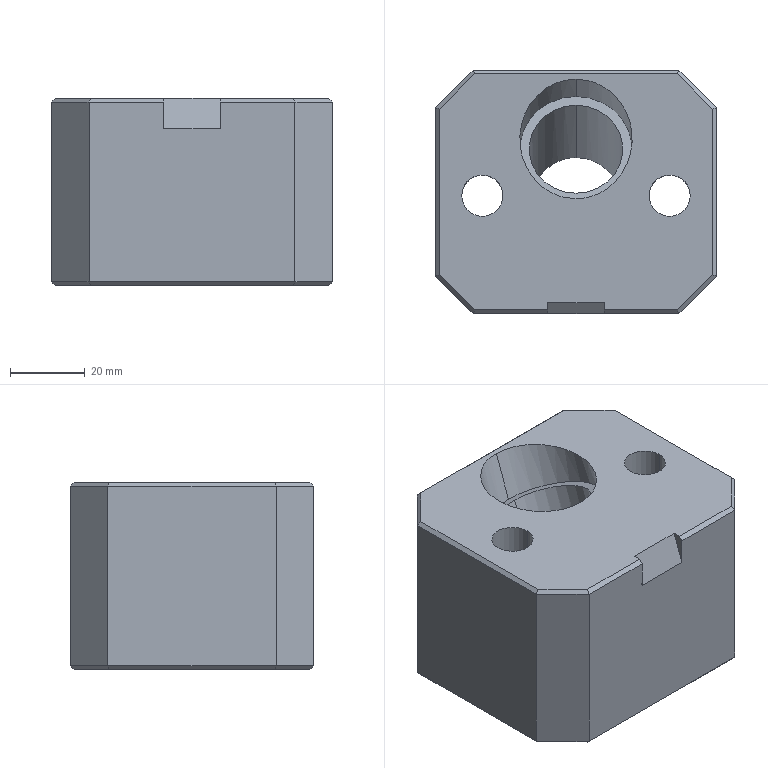Part | Creo | 3 solids | 49 faces | box 75 x 65 x 50 mm | volume 192479 mm3 | plane 33 | cylinder 16 | commonest cylinder face diameters 11 x4 18 x4 11.98 x2 12 x2 25 x2 30 x2
STEP:
#1=CARTESIAN_POINT('',(0.,-322.338,40.));
#2=VERTEX_POINT('',#1);
#3=CARTESIAN_POINT('',(0.,-290.412,40.));
#4=VERTEX_POINT('',#3);
#5=CARTESIAN_POINT('',(0.,-322.338,40.));
#6=CARTESIAN_POINT('',(-1.768,-322.338,40.));
#7=CARTESIAN_POINT('',(-5.588,-321.656,40.));
#8=CARTESIAN_POINT('',(-10.029,-318.608,40.));
#9=CARTESIAN_POINT('',(-12.65,-315.161,40.));
#10=CARTESIAN_POINT('',(-14.047,-312.268,40.));
#11=CARTESIAN_POINT('',(-14.71,-309.769,40.));
#12=CARTESIAN_POINT('',(-14.961,-307.801,40.));
#13=CARTESIAN_POINT('',(-15.02,-306.375,40.));
#14=CARTESIAN_POINT('',(-14.961,-304.949,40.));
#15=CARTESIAN_POINT('',(-14.71,-302.981,40.));
#16=CARTESIAN_POINT('',(-14.047,-300.481,40.));
#17=CARTESIAN_POINT('',(-12.65,-297.589,40.));
#18=CARTESIAN_POINT('',(-10.029,-294.142,40.));
#19=CARTESIAN_POINT('',(-5.588,-291.094,40.));
#20=CARTESIAN_POINT('',(-1.768,-290.412,40.));
#21=CARTESIAN_POINT('',(0.,-290.412,40.));
#22=B_SPLINE_CURVE_WITH_KNOTS('',3,(#5,#6,#7,#8,#9,#10,#11,#12,#13,#14,#15,#16,#17,#18,#19,#20,#21),.UNSPECIFIED.,.F.,.F.,(4,1,1,1,1,1,1,1,1,1,1,1,1,1,4),(0.,0.125,0.25,0.3125,0.375,0.4375,0.4688,0.5,0.5312,0.5625,0.625,0.6875,0.75,0.875,1.),.UNSPECIFIED.);
#23=EDGE_CURVE('',#2,#4,#22,.T.);
#24=ORIENTED_EDGE('',*,*,#23,.T.);
#25=CARTESIAN_POINT('',(0.,-295.009,27.371));
#26=VERTEX_POINT('',#25);
#27=CARTESIAN_POINT('',(0.,-290.412,40.));
#28=DIRECTION('',(0.,-0.342,-0.9397));
#29=VECTOR('',#28,13.44);
#30=LINE('',#27,#29);
#31=EDGE_CURVE('',#4,#26,#30,.T.);
#32=ORIENTED_EDGE('',*,*,#31,.T.);
#33=CARTESIAN_POINT('',(0.,-323.2,37.631));
#34=VERTEX_POINT('',#33);
#35=CARTESIAN_POINT('',(0.,-309.104,32.501));
#36=DIRECTION('',(0.,0.342,0.9397));
#37=DIRECTION('',(0.,0.9397,-0.342));
#38=AXIS2_PLACEMENT_3D('',#35,#36,#37);
#39=CIRCLE('',#38,15.);
#40=EDGE_CURVE('',#26,#34,#39,.T.);
#41=ORIENTED_EDGE('',*,*,#40,.T.);
#42=CARTESIAN_POINT('',(0.,-322.338,40.));
#43=DIRECTION('',(0.,-0.342,-0.9397));
#44=VECTOR('',#43,2.521);
#45=LINE('',#42,#44);
#46=EDGE_CURVE('',#2,#34,#45,.T.);
#47=ORIENTED_EDGE('',*,*,#46,.F.);
#48=EDGE_LOOP('',(#24,#32,#41,#47));
#49=FACE_OUTER_BOUND('',#48,.F.);
#50=CARTESIAN_POINT('',(0.,-302.52,50.59));
#51=DIRECTION('',(0.,-0.342,-0.9397));
#52=DIRECTION('',(0.,-0.9397,0.342));
#53=AXIS2_PLACEMENT_3D('',#50,#51,#52);
#54=CYLINDRICAL_SURFACE('',#53,15.);
#55=ADVANCED_FACE('',(#49),#54,.F.);
#56=CARTESIAN_POINT('',(-7.502,-352.,40.));
#57=VERTEX_POINT('',#56);
#58=CARTESIAN_POINT('',(-7.502,-350.064,40.));
#59=VERTEX_POINT('',#58);
#60=CARTESIAN_POINT('',(-7.502,-352.,40.));
#61=DIRECTION('',(0.,1.,0.));
#62=VECTOR('',#61,1.936);
#63=LINE('',#60,#62);
#64=EDGE_CURVE('',#57,#59,#63,.T.);
#65=ORIENTED_EDGE('',*,*,#64,.F.);
#66=CARTESIAN_POINT('',(-27.087,-352.,40.));
#67=VERTEX_POINT('',#66);
#68=CARTESIAN_POINT('',(-7.502,-352.,40.));
#69=DIRECTION('',(-1.,0.,0.));
#70=VECTOR('',#69,19.586);
#71=LINE('',#68,#70);
#72=EDGE_CURVE('',#57,#67,#71,.T.);
#73=ORIENTED_EDGE('',*,*,#72,.T.);
#74=CARTESIAN_POINT('',(-36.502,-342.586,40.));
#75=VERTEX_POINT('',#74);
#76=CARTESIAN_POINT('',(-36.502,-342.586,40.));
#77=DIRECTION('',(0.7071,-0.7071,0.));
#78=VECTOR('',#77,13.314);
#79=LINE('',#76,#78);
#80=EDGE_CURVE('',#75,#67,#79,.T.);
#81=ORIENTED_EDGE('',*,*,#80,.F.);
#82=CARTESIAN_POINT('',(-36.502,-298.414,40.));
#83=VERTEX_POINT('',#82);
#84=CARTESIAN_POINT('',(-36.502,-342.586,40.));
#85=DIRECTION('',(0.,1.,0.));
#86=VECTOR('',#85,44.172);
#87=LINE('',#84,#86);
#88=EDGE_CURVE('',#75,#83,#87,.T.);
#89=ORIENTED_EDGE('',*,*,#88,.T.);
#90=CARTESIAN_POINT('',(-27.087,-289.,40.));
#91=VERTEX_POINT('',#90);
#92=CARTESIAN_POINT('',(-27.087,-289.,40.));
#93=DIRECTION('',(-0.7071,-0.7071,0.));
#94=VECTOR('',#93,13.314);
#95=LINE('',#92,#94);
#96=EDGE_CURVE('',#91,#83,#95,.T.);
#97=ORIENTED_EDGE('',*,*,#96,.F.);
#98=CARTESIAN_POINT('',(27.084,-289.,40.));
#99=VERTEX_POINT('',#98);
#100=CARTESIAN_POINT('',(-27.087,-289.,40.));
#101=DIRECTION('',(1.,0.,0.));
#102=VECTOR('',#101,54.172);
#103=LINE('',#100,#102);
#104=EDGE_CURVE('',#91,#99,#103,.T.);
#105=ORIENTED_EDGE('',*,*,#104,.T.);
#106=CARTESIAN_POINT('',(36.498,-298.414,40.));
#107=VERTEX_POINT('',#106);
#108=CARTESIAN_POINT('',(36.498,-298.414,40.));
#109=DIRECTION('',(-0.7071,0.7071,0.));
#110=VECTOR('',#109,13.314);
#111=LINE('',#108,#110);
#112=EDGE_CURVE('',#107,#99,#111,.T.);
#113=ORIENTED_EDGE('',*,*,#112,.F.);
#114=CARTESIAN_POINT('',(36.498,-342.586,40.));
#115=VERTEX_POINT('',#114);
#116=CARTESIAN_POINT('',(36.498,-298.414,40.));
#117=DIRECTION('',(0.,-1.,0.));
#118=VECTOR('',#117,44.172);
#119=LINE('',#116,#118);
#120=EDGE_CURVE('',#107,#115,#119,.T.);
#121=ORIENTED_EDGE('',*,*,#120,.T.);
#122=CARTESIAN_POINT('',(27.084,-352.,40.));
#123=VERTEX_POINT('',#122);
#124=CARTESIAN_POINT('',(27.084,-352.,40.));
#125=DIRECTION('',(0.7071,0.7071,0.));
#126=VECTOR('',#125,13.314);
#127=LINE('',#124,#126);
#128=EDGE_CURVE('',#123,#115,#127,.T.);
#129=ORIENTED_EDGE('',*,*,#128,.F.);
#130=CARTESIAN_POINT('',(7.498,-352.,40.));
#131=VERTEX_POINT('',#130);
#132=CARTESIAN_POINT('',(27.084,-352.,40.));
#133=DIRECTION('',(-1.,0.,0.));
#134=VECTOR('',#133,19.586);
#135=LINE('',#132,#134);
#136=EDGE_CURVE('',#123,#131,#135,.T.);
#137=ORIENTED_EDGE('',*,*,#136,.T.);
#138=CARTESIAN_POINT('',(7.498,-350.064,40.));
#139=VERTEX_POINT('',#138);
#140=CARTESIAN_POINT('',(7.498,-350.064,40.));
#141=DIRECTION('',(0.,-1.,0.));
#142=VECTOR('',#141,1.936);
#143=LINE('',#140,#142);
#144=EDGE_CURVE('',#139,#131,#143,.T.);
#145=ORIENTED_EDGE('',*,*,#144,.F.);
#146=CARTESIAN_POINT('',(-7.502,-350.064,40.));
#147=DIRECTION('',(1.,0.,0.));
#148=VECTOR('',#147,15.);
#149=LINE('',#146,#148);
#150=EDGE_CURVE('',#59,#139,#149,.T.);
#151=ORIENTED_EDGE('',*,*,#150,.F.);
#152=EDGE_LOOP('',(#65,#73,#81,#89,#97,#105,#113,#121,#129,#137,#145,#151));
#153=FACE_OUTER_BOUND('',#152,.F.);
#154=CARTESIAN_POINT('',(-19.502,-321.5,40.));
#155=VERTEX_POINT('',#154);
#156=CARTESIAN_POINT('',(-30.502,-321.5,40.));
#157=VERTEX_POINT('',#156);
#158=CARTESIAN_POINT('',(-25.002,-321.5,40.));
#159=DIRECTION('',(0.,0.,-1.));
#160=DIRECTION('',(1.,0.,0.));
#161=AXIS2_PLACEMENT_3D('',#158,#159,#160);
#162=CIRCLE('',#161,5.5);
#163=EDGE_CURVE('',#155,#157,#162,.T.);
#164=ORIENTED_EDGE('',*,*,#163,.F.);
#165=CARTESIAN_POINT('',(-25.002,-321.5,40.));
#166=DIRECTION('',(0.,0.,-1.));
#167=DIRECTION('',(-1.,0.,0.));
#168=AXIS2_PLACEMENT_3D('',#165,#166,#167);
#169=CIRCLE('',#168,5.5);
#170=EDGE_CURVE('',#157,#155,#169,.T.);
#171=ORIENTED_EDGE('',*,*,#170,.F.);
#172=EDGE_LOOP('',(#164,#171));
#173=FACE_BOUND('',#172,.F.);
#174=CARTESIAN_POINT('',(30.498,-321.5,40.));
#175=VERTEX_POINT('',#174);
#176=CARTESIAN_POINT('',(19.498,-321.5,40.));
#177=VERTEX_POINT('',#176);
#178=CARTESIAN_POINT('',(24.998,-321.5,40.));
#179=DIRECTION('',(0.,0.,-1.));
#180=DIRECTION('',(1.,0.,0.));
#181=AXIS2_PLACEMENT_3D('',#178,#179,#180);
#182=CIRCLE('',#181,5.5);
#183=EDGE_CURVE('',#175,#177,#182,.T.);
#184=ORIENTED_EDGE('',*,*,#183,.F.);
#185=CARTESIAN_POINT('',(24.998,-321.5,40.));
#186=DIRECTION('',(0.,0.,-1.));
#187=DIRECTION('',(-1.,0.,0.));
#188=AXIS2_PLACEMENT_3D('',#185,#186,#187);
#189=CIRCLE('',#188,5.5);
#190=EDGE_CURVE('',#177,#175,#189,.T.);
#191=ORIENTED_EDGE('',*,*,#190,.F.);
#192=EDGE_LOOP('',(#184,#191));
#193=FACE_BOUND('',#192,.F.);
#194=ORIENTED_EDGE('',*,*,#23,.F.);
#195=CARTESIAN_POINT('',(0.,-290.412,40.));
#196=CARTESIAN_POINT('',(1.768,-290.412,40.));
#197=CARTESIAN_POINT('',(5.588,-291.094,40.));
#198=CARTESIAN_POINT('',(10.029,-294.142,40.));
#199=CARTESIAN_POINT('',(12.65,-297.589,40.));
#200=CARTESIAN_POINT('',(14.047,-300.481,40.));
#201=CARTESIAN_POINT('',(14.71,-302.981,40.));
#202=CARTESIAN_POINT('',(14.961,-304.949,40.));
#203=CARTESIAN_POINT('',(15.02,-306.375,40.));
#204=CARTESIAN_POINT('',(14.961,-307.801,40.));
#205=CARTESIAN_POINT('',(14.71,-309.769,40.));
#206=CARTESIAN_POINT('',(14.047,-312.268,40.));
#207=CARTESIAN_POINT('',(12.65,-315.161,40.));
#208=CARTESIAN_POINT('',(10.029,-318.608,40.));
#209=CARTESIAN_POINT('',(5.588,-321.656,40.));
#210=CARTESIAN_POINT('',(1.768,-322.338,40.));
#211=CARTESIAN_POINT('',(0.,-322.338,40.));
#212=B_SPLINE_CURVE_WITH_KNOTS('',3,(#195,#196,#197,#198,#199,#200,#201,#202,#203,#204,#205,#206,#207,#208,#209,#210,#211),.UNSPECIFIED.,.F.,.F.,(4,1,1,1,1,1,1,1,1,1,1,1,1,1,4),(0.,0.125,0.25,0.3125,0.375,0.4375,0.4688,0.5,0.5312,0.5625,0.625,0.6875,0.75,0.875,1.),.UNSPECIFIED.);
#213=EDGE_CURVE('',#4,#2,#212,.T.);
#214=ORIENTED_EDGE('',*,*,#213,.F.);
#215=EDGE_LOOP('',(#194,#214));
#216=FACE_BOUND('',#215,.F.);
#217=CARTESIAN_POINT('',(365.934,-307.397,40.));
#218=DIRECTION('',(0.,0.,1.));
#219=DIRECTION('',(-1.,0.,0.));
#220=AXIS2_PLACEMENT_3D('',#217,#218,#219);
#221=PLANE('',#220);
#222=ADVANCED_FACE('',(#153,#173,#193,#216),#221,.T.);
#223=ORIENTED_EDGE('',*,*,#64,.T.);
#224=CARTESIAN_POINT('',(-7.502,-353.,31.933));
#225=VERTEX_POINT('',#224);
#226=CARTESIAN_POINT('',(-7.502,-353.,31.933));
#227=DIRECTION('',(0.,0.342,0.9397));
#228=VECTOR('',#227,8.584);
#229=LINE('',#226,#228);
#230=EDGE_CURVE('',#225,#59,#229,.T.);
#231=ORIENTED_EDGE('',*,*,#230,.F.);
#232=CARTESIAN_POINT('',(-7.502,-353.,39.));
#233=VERTEX_POINT('',#232);
#234=CARTESIAN_POINT('',(-7.502,-353.,31.933));
#235=DIRECTION('',(0.,0.,1.));
#236=VECTOR('',#235,7.067);
#237=LINE('',#234,#236);
#238=EDGE_CURVE('',#225,#233,#237,.T.);
#239=ORIENTED_EDGE('',*,*,#238,.T.);
#240=CARTESIAN_POINT('',(-7.502,-352.,40.));
#241=DIRECTION('',(0.,-0.7071,-0.7071));
#242=VECTOR('',#241,1.414);
#243=LINE('',#240,#242);
#244=EDGE_CURVE('',#57,#233,#243,.T.);
#245=ORIENTED_EDGE('',*,*,#244,.F.);
#246=EDGE_LOOP('',(#223,#231,#239,#245));
#247=FACE_OUTER_BOUND('',#246,.F.);
#248=CARTESIAN_POINT('',(-7.502,-370.58,-2.601));
#249=DIRECTION('',(-1.,0.,0.));
#250=DIRECTION('',(0.,0.,1.));
#251=AXIS2_PLACEMENT_3D('',#248,#249,#250);
#252=PLANE('',#251);
#253=ADVANCED_FACE('',(#247),#252,.F.);
#254=ORIENTED_EDGE('',*,*,#150,.T.);
#255=CARTESIAN_POINT('',(7.498,-353.,31.933));
#256=VERTEX_POINT('',#255);
#257=CARTESIAN_POINT('',(7.498,-350.064,40.));
#258=DIRECTION('',(0.,-0.342,-0.9397));
#259=VECTOR('',#258,8.584);
#260=LINE('',#257,#259);
#261=EDGE_CURVE('',#139,#256,#260,.T.);
#262=ORIENTED_EDGE('',*,*,#261,.T.);
#263=CARTESIAN_POINT('',(7.498,-353.,31.933));
#264=DIRECTION('',(-1.,0.,0.));
#265=VECTOR('',#264,15.);
#266=LINE('',#263,#265);
#267=EDGE_CURVE('',#256,#225,#266,.T.);
#268=ORIENTED_EDGE('',*,*,#267,.T.);
#269=ORIENTED_EDGE('',*,*,#230,.T.);
#270=EDGE_LOOP('',(#254,#262,#268,#269));
#271=FACE_OUTER_BOUND('',#270,.F.);
#272=CARTESIAN_POINT('',(-0.00154,-366.156,-4.212));
#273=DIRECTION('',(0.,0.9397,-0.342));
#274=DIRECTION('',(0.,0.342,0.9397));
#275=AXIS2_PLACEMENT_3D('',#272,#273,#274);
#276=PLANE('',#275);
#277=ADVANCED_FACE('',(#271),#276,.F.);
#278=ORIENTED_EDGE('',*,*,#144,.T.);
#279=CARTESIAN_POINT('',(7.498,-353.,39.));
#280=VERTEX_POINT('',#279);
#281=CARTESIAN_POINT('',(7.498,-353.,39.));
#282=DIRECTION('',(0.,0.7071,0.7071));
#283=VECTOR('',#282,1.414);
#284=LINE('',#281,#283);
#285=EDGE_CURVE('',#280,#131,#284,.T.);
#286=ORIENTED_EDGE('',*,*,#285,.F.);
#287=CARTESIAN_POINT('',(7.498,-353.,39.));
#288=DIRECTION('',(0.,0.,-1.));
#289=VECTOR('',#288,7.067);
#290=LINE('',#287,#289);
#291=EDGE_CURVE('',#280,#256,#290,.T.);
#292=ORIENTED_EDGE('',*,*,#291,.T.);
#293=ORIENTED_EDGE('',*,*,#261,.F.);
#294=EDGE_LOOP('',(#278,#286,#292,#293));
#295=FACE_OUTER_BOUND('',#294,.F.);
#296=CARTESIAN_POINT('',(7.498,-370.58,-2.601));
#297=DIRECTION('',(1.,0.,0.));
#298=DIRECTION('',(0.,0.,-1.));
#299=AXIS2_PLACEMENT_3D('',#296,#297,#298);
#300=PLANE('',#299);
#301=ADVANCED_FACE('',(#295),#300,.F.);
#302=ORIENTED_EDGE('',*,*,#285,.T.);
#303=ORIENTED_EDGE('',*,*,#136,.F.);
#304=CARTESIAN_POINT('',(27.498,-353.,39.));
#305=VERTEX_POINT('',#304);
#306=CARTESIAN_POINT('',(27.498,-353.,39.));
#307=DIRECTION('',(-0.2811,0.6786,0.6786));
#308=VECTOR('',#307,1.474);
#309=LINE('',#306,#308);
#310=EDGE_CURVE('',#305,#123,#309,.T.);
#311=ORIENTED_EDGE('',*,*,#310,.F.);
#312=CARTESIAN_POINT('',(7.498,-353.,39.));
#313=DIRECTION('',(1.,0.,0.));
#314=VECTOR('',#313,20.);
#315=LINE('',#312,#314);
#316=EDGE_CURVE('',#280,#305,#315,.T.);
#317=ORIENTED_EDGE('',*,*,#316,.F.);
#318=EDGE_LOOP('',(#302,#303,#311,#317));
#319=FACE_OUTER_BOUND('',#318,.F.);
#320=CARTESIAN_POINT('',(365.934,-352.,40.));
#321=DIRECTION('',(0.,0.7071,-0.7071));
#322=DIRECTION('',(1.,0.,0.));
#323=AXIS2_PLACEMENT_3D('',#320,#321,#322);
#324=PLANE('',#323);
#325=ADVANCED_FACE('',(#319),#324,.F.);
#326=ORIENTED_EDGE('',*,*,#128,.T.);
#327=CARTESIAN_POINT('',(37.498,-343.,39.));
#328=VERTEX_POINT('',#327);
#329=CARTESIAN_POINT('',(37.498,-343.,39.));
#330=DIRECTION('',(-0.6786,0.2811,0.6786));
#331=VECTOR('',#330,1.474);
#332=LINE('',#329,#331);
#333=EDGE_CURVE('',#328,#115,#332,.T.);
#334=ORIENTED_EDGE('',*,*,#333,.F.);
#335=CARTESIAN_POINT('',(27.498,-353.,39.));
#336=DIRECTION('',(0.7071,0.7071,0.));
#337=VECTOR('',#336,14.142);
#338=LINE('',#335,#337);
#339=EDGE_CURVE('',#305,#328,#338,.T.);
#340=ORIENTED_EDGE('',*,*,#339,.F.);
#341=ORIENTED_EDGE('',*,*,#310,.T.);
#342=EDGE_LOOP('',(#326,#334,#340,#341));
#343=FACE_OUTER_BOUND('',#342,.F.);
#344=CARTESIAN_POINT('',(218.811,-160.274,40.));
#345=DIRECTION('',(-0.5,0.5,-0.7071));
#346=DIRECTION('',(0.7071,0.7071,0.));
#347=AXIS2_PLACEMENT_3D('',#344,#345,#346);
#348=PLANE('',#347);
#349=ADVANCED_FACE('',(#343),#348,.F.);
#350=ORIENTED_EDGE('',*,*,#333,.T.);
#351=ORIENTED_EDGE('',*,*,#120,.F.);
#352=CARTESIAN_POINT('',(37.498,-298.,39.));
#353=VERTEX_POINT('',#352);
#354=CARTESIAN_POINT('',(37.498,-298.,39.));
#355=DIRECTION('',(-0.6786,-0.2811,0.6786));
#356=VECTOR('',#355,1.474);
#357=LINE('',#354,#356);
#358=EDGE_CURVE('',#353,#107,#357,.T.);
#359=ORIENTED_EDGE('',*,*,#358,.F.);
#360=CARTESIAN_POINT('',(37.498,-343.,39.));
#361=DIRECTION('',(0.,1.,0.));
#362=VECTOR('',#361,45.);
#363=LINE('',#360,#362);
#364=EDGE_CURVE('',#328,#353,#363,.T.);
#365=ORIENTED_EDGE('',*,*,#364,.F.);
#366=EDGE_LOOP('',(#350,#351,#359,#365));
#367=FACE_OUTER_BOUND('',#366,.F.);
#368=CARTESIAN_POINT('',(36.498,-307.397,40.));
#369=DIRECTION('',(0.7071,0.,0.7071));
#370=DIRECTION('',(0.,-1.,0.));
#371=AXIS2_PLACEMENT_3D('',#368,#369,#370);
#372=PLANE('',#371);
#373=ADVANCED_FACE('',(#367),#372,.T.);
#374=ORIENTED_EDGE('',*,*,#358,.T.);
#375=ORIENTED_EDGE('',*,*,#112,.T.);
#376=CARTESIAN_POINT('',(27.498,-288.,39.));
#377=VERTEX_POINT('',#376);
#378=CARTESIAN_POINT('',(27.498,-288.,39.));
#379=DIRECTION('',(-0.2811,-0.6786,0.6786));
#380=VECTOR('',#379,1.474);
#381=LINE('',#378,#380);
#382=EDGE_CURVE('',#377,#99,#381,.T.);
#383=ORIENTED_EDGE('',*,*,#382,.F.);
#384=CARTESIAN_POINT('',(37.498,-298.,39.));
#385=DIRECTION('',(-0.7071,0.7071,0.));
#386=VECTOR('',#385,14.142);
#387=LINE('',#384,#386);
#388=EDGE_CURVE('',#353,#377,#387,.T.);
#389=ORIENTED_EDGE('',*,*,#388,.F.);
#390=EDGE_LOOP('',(#374,#375,#383,#389));
#391=FACE_OUTER_BOUND('',#390,.F.);
#392=CARTESIAN_POINT('',(205.708,-467.624,40.));
#393=DIRECTION('',(-0.5,-0.5,-0.7071));
#394=DIRECTION('',(-0.7071,0.7071,0.));
#395=AXIS2_PLACEMENT_3D('',#392,#393,#394);
#396=PLANE('',#395);
#397=ADVANCED_FACE('',(#391),#396,.F.);
#398=CARTESIAN_POINT('',(-27.502,-288.,39.));
#399=VERTEX_POINT('',#398);
#400=CARTESIAN_POINT('',(-27.502,-288.,39.));
#401=DIRECTION('',(0.2811,-0.6786,0.6786));
#402=VECTOR('',#401,1.474);
#403=LINE('',#400,#402);
#404=EDGE_CURVE('',#399,#91,#403,.T.);
#405=ORIENTED_EDGE('',*,*,#404,.F.);
#406=CARTESIAN_POINT('',(27.498,-288.,39.));
#407=DIRECTION('',(-1.,0.,0.));
#408=VECTOR('',#407,55.);
#409=LINE('',#406,#408);
#410=EDGE_CURVE('',#377,#399,#409,.T.);
#411=ORIENTED_EDGE('',*,*,#410,.F.);
#412=ORIENTED_EDGE('',*,*,#382,.T.);
#413=ORIENTED_EDGE('',*,*,#104,.F.);
#414=EDGE_LOOP('',(#405,#411,#412,#413));
#415=FACE_OUTER_BOUND('',#414,.F.);
#416=CARTESIAN_POINT('',(278.498,-288.,39.));
#417=DIRECTION('',(0.,-0.7071,-0.7071));
#418=DIRECTION('',(1.,0.,0.));
#419=AXIS2_PLACEMENT_3D('',#416,#417,#418);
#420=PLANE('',#419);
#421=ADVANCED_FACE('',(#415),#420,.F.);
#422=ORIENTED_EDGE('',*,*,#404,.T.);
#423=ORIENTED_EDGE('',*,*,#96,.T.);
#424=CARTESIAN_POINT('',(-37.502,-298.,39.));
#425=VERTEX_POINT('',#424);
#426=CARTESIAN_POINT('',(-36.502,-298.414,40.));
#427=DIRECTION('',(-0.6786,0.2811,-0.6786));
#428=VECTOR('',#427,1.474);
#429=LINE('',#426,#428);
#430=EDGE_CURVE('',#83,#425,#429,.T.);
#431=ORIENTED_EDGE('',*,*,#430,.T.);
#432=CARTESIAN_POINT('',(-27.502,-288.,39.));
#433=DIRECTION('',(-0.7071,-0.7071,0.));
#434=VECTOR('',#433,14.142);
#435=LINE('',#432,#434);
#436=EDGE_CURVE('',#399,#425,#435,.T.);
#437=ORIENTED_EDGE('',*,*,#436,.F.);
#438=EDGE_LOOP('',(#422,#423,#431,#437));
#439=FACE_OUTER_BOUND('',#438,.F.);
#440=CARTESIAN_POINT('',(160.225,-101.688,40.));
#441=DIRECTION('',(-0.5,0.5,0.7071));
#442=DIRECTION('',(0.7071,0.7071,0.));
#443=AXIS2_PLACEMENT_3D('',#440,#441,#442);
#444=PLANE('',#443);
#445=ADVANCED_FACE('',(#439),#444,.T.);
#446=CARTESIAN_POINT('',(-37.502,-343.,39.));
#447=VERTEX_POINT('',#446);
#448=CARTESIAN_POINT('',(-36.502,-342.586,40.));
#449=DIRECTION('',(-0.6786,-0.2811,-0.6786));
#450=VECTOR('',#449,1.474);
#451=LINE('',#448,#450);
#452=EDGE_CURVE('',#75,#447,#451,.T.);
#453=ORIENTED_EDGE('',*,*,#452,.T.);
#454=CARTESIAN_POINT('',(-37.502,-298.,39.));
#455=DIRECTION('',(0.,-1.,0.));
#456=VECTOR('',#455,45.);
#457=LINE('',#454,#456);
#458=EDGE_CURVE('',#425,#447,#457,.T.);
#459=ORIENTED_EDGE('',*,*,#458,.F.);
#460=ORIENTED_EDGE('',*,*,#430,.F.);
#461=ORIENTED_EDGE('',*,*,#88,.F.);
#462=EDGE_LOOP('',(#453,#459,#460,#461));
#463=FACE_OUTER_BOUND('',#462,.F.);
#464=CARTESIAN_POINT('',(-36.502,-307.397,40.));
#465=DIRECTION('',(0.7071,0.,-0.7071));
#466=DIRECTION('',(0.,-1.,0.));
#467=AXIS2_PLACEMENT_3D('',#464,#465,#466);
#468=PLANE('',#467);
#469=ADVANCED_FACE('',(#463),#468,.F.);
#470=CARTESIAN_POINT('',(-27.502,-353.,39.));
#471=VERTEX_POINT('',#470);
#472=CARTESIAN_POINT('',(-37.502,-343.,39.));
#473=DIRECTION('',(0.7071,-0.7071,0.));
#474=VECTOR('',#473,14.142);
#475=LINE('',#472,#474);
#476=EDGE_CURVE('',#447,#471,#475,.T.);
#477=ORIENTED_EDGE('',*,*,#476,.F.);
#478=ORIENTED_EDGE('',*,*,#452,.F.);
#479=ORIENTED_EDGE('',*,*,#80,.T.);
#480=CARTESIAN_POINT('',(-27.087,-352.,40.));
#481=DIRECTION('',(-0.2811,-0.6786,-0.6786));
#482=VECTOR('',#481,1.474);
#483=LINE('',#480,#482);
#484=EDGE_CURVE('',#67,#471,#483,.T.);
#485=ORIENTED_EDGE('',*,*,#484,.T.);
#486=EDGE_LOOP('',(#477,#478,#479,#485));
#487=FACE_OUTER_BOUND('',#486,.F.);
#488=CARTESIAN_POINT('',(147.122,-526.21,40.));
#489=DIRECTION('',(-0.5,-0.5,0.7071));
#490=DIRECTION('',(-0.7071,0.7071,0.));
#491=AXIS2_PLACEMENT_3D('',#488,#489,#490);
#492=PLANE('',#491);
#493=ADVANCED_FACE('',(#487),#492,.T.);
#494=CARTESIAN_POINT('',(-27.502,-353.,-9.));
#495=VERTEX_POINT('',#494);
#496=CARTESIAN_POINT('',(-27.502,-353.,-9.));
#497=DIRECTION('',(0.,0.,1.));
#498=VECTOR('',#497,48.);
#499=LINE('',#496,#498);
#500=EDGE_CURVE('',#495,#471,#499,.T.);
#501=ORIENTED_EDGE('',*,*,#500,.F.);
#502=CARTESIAN_POINT('',(-37.502,-343.,-9.));
#503=VERTEX_POINT('',#502);
#504=CARTESIAN_POINT('',(-27.502,-353.,-9.));
#505=DIRECTION('',(-0.7071,0.7071,0.));
#506=VECTOR('',#505,14.142);
#507=LINE('',#504,#506);
#508=EDGE_CURVE('',#495,#503,#507,.T.);
#509=ORIENTED_EDGE('',*,*,#508,.T.);
#510=CARTESIAN_POINT('',(-37.502,-343.,39.));
#511=DIRECTION('',(0.,0.,-1.));
#512=VECTOR('',#511,48.);
#513=LINE('',#510,#512);
#514=EDGE_CURVE('',#447,#503,#513,.T.);
#515=ORIENTED_EDGE('',*,*,#514,.F.);
#516=ORIENTED_EDGE('',*,*,#476,.T.);
#517=EDGE_LOOP('',(#501,#509,#515,#516));
#518=FACE_OUTER_BOUND('',#517,.F.);
#519=CARTESIAN_POINT('',(-27.502,-353.,-20.39));
#520=DIRECTION('',(0.7071,0.7071,0.));
#521=DIRECTION('',(0.,0.,-1.));
#522=AXIS2_PLACEMENT_3D('',#519,#520,#521);
#523=PLANE('',#522);
#524=ADVANCED_FACE('',(#518),#523,.F.);
#525=ORIENTED_EDGE('',*,*,#238,.F.);
#526=ORIENTED_EDGE('',*,*,#267,.F.);
#527=ORIENTED_EDGE('',*,*,#291,.F.);
#528=ORIENTED_EDGE('',*,*,#316,.T.);
#529=CARTESIAN_POINT('',(27.498,-353.,-9.));
#530=VERTEX_POINT('',#529);
#531=CARTESIAN_POINT('',(27.498,-353.,39.));
#532=DIRECTION('',(0.,0.,-1.));
#533=VECTOR('',#532,48.);
#534=LINE('',#531,#533);
#535=EDGE_CURVE('',#305,#530,#534,.T.);
#536=ORIENTED_EDGE('',*,*,#535,.T.);
#537=CARTESIAN_POINT('',(27.498,-353.,-9.));
#538=DIRECTION('',(-1.,0.,0.));
#539=VECTOR('',#538,55.);
#540=LINE('',#537,#539);
#541=EDGE_CURVE('',#530,#495,#540,.T.);
#542=ORIENTED_EDGE('',*,*,#541,.T.);
#543=ORIENTED_EDGE('',*,*,#500,.T.);
#544=CARTESIAN_POINT('',(-27.502,-353.,39.));
#545=DIRECTION('',(1.,0.,0.));
#546=VECTOR('',#545,20.);
#547=LINE('',#544,#546);
#548=EDGE_CURVE('',#471,#233,#547,.T.);
#549=ORIENTED_EDGE('',*,*,#548,.T.);
#550=EDGE_LOOP('',(#525,#526,#527,#528,#536,#542,#543,#549));
#551=FACE_OUTER_BOUND('',#550,.F.);
#552=CARTESIAN_POINT('',(189.995,-353.,-20.39));
#553=DIRECTION('',(0.,-1.,0.));
#554=DIRECTION('',(0.,0.,-1.));
#555=AXIS2_PLACEMENT_3D('',#552,#553,#554);
#556=PLANE('',#555);
#557=ADVANCED_FACE('',(#551),#556,.T.);
#558=ORIENTED_EDGE('',*,*,#339,.T.);
#559=CARTESIAN_POINT('',(37.498,-343.,-9.));
#560=VERTEX_POINT('',#559);
#561=CARTESIAN_POINT('',(37.498,-343.,-9.));
#562=DIRECTION('',(0.,0.,1.));
#563=VECTOR('',#562,48.);
#564=LINE('',#561,#563);
#565=EDGE_CURVE('',#560,#328,#564,.T.);
#566=ORIENTED_EDGE('',*,*,#565,.F.);
#567=CARTESIAN_POINT('',(37.498,-343.,-9.));
#568=DIRECTION('',(-0.7071,-0.7071,0.));
#569=VECTOR('',#568,14.142);
#570=LINE('',#567,#569);
#571=EDGE_CURVE('',#560,#530,#570,.T.);
#572=ORIENTED_EDGE('',*,*,#571,.T.);
#573=ORIENTED_EDGE('',*,*,#535,.F.);
#574=EDGE_LOOP('',(#558,#566,#572,#573));
#575=FACE_OUTER_BOUND('',#574,.F.);
#576=CARTESIAN_POINT('',(37.498,-343.,-66.89));
#577=DIRECTION('',(0.7071,-0.7071,0.));
#578=DIRECTION('',(0.,0.,1.));
#579=AXIS2_PLACEMENT_3D('',#576,#577,#578);
#580=PLANE('',#579);
#581=ADVANCED_FACE('',(#575),#580,.T.);
#582=CARTESIAN_POINT('',(37.498,-298.,-9.));
#583=VERTEX_POINT('',#582);
#584=CARTESIAN_POINT('',(37.498,-298.,-9.));
#585=DIRECTION('',(0.,-1.,0.));
#586=VECTOR('',#585,45.);
#587=LINE('',#584,#586);
#588=EDGE_CURVE('',#583,#560,#587,.T.);
#589=ORIENTED_EDGE('',*,*,#588,.T.);
#590=ORIENTED_EDGE('',*,*,#565,.T.);
#591=ORIENTED_EDGE('',*,*,#364,.T.);
#592=CARTESIAN_POINT('',(37.498,-298.,39.));
#593=DIRECTION('',(0.,0.,-1.));
#594=VECTOR('',#593,48.);
#595=LINE('',#592,#594);
#596=EDGE_CURVE('',#353,#583,#595,.T.);
#597=ORIENTED_EDGE('',*,*,#596,.T.);
#598=EDGE_LOOP('',(#589,#590,#591,#597));
#599=FACE_OUTER_BOUND('',#598,.F.);
#600=CARTESIAN_POINT('',(37.498,-339.116,-66.89));
#601=DIRECTION('',(-1.,0.,0.));
#602=DIRECTION('',(0.,0.,1.));
#603=AXIS2_PLACEMENT_3D('',#600,#601,#602);
#604=PLANE('',#603);
#605=ADVANCED_FACE('',(#599),#604,.F.);
#606=CARTESIAN_POINT('',(36.498,-342.586,-10.));
#607=VERTEX_POINT('',#606);
#608=CARTESIAN_POINT('',(36.498,-298.414,-10.));
#609=VERTEX_POINT('',#608);
#610=CARTESIAN_POINT('',(36.498,-342.586,-10.));
#611=DIRECTION('',(0.,1.,0.));
#612=VECTOR('',#611,44.172);
#613=LINE('',#610,#612);
#614=EDGE_CURVE('',#607,#609,#613,.T.);
#615=ORIENTED_EDGE('',*,*,#614,.F.);
#616=CARTESIAN_POINT('',(37.498,-343.,-9.));
#617=DIRECTION('',(-0.6786,0.2811,-0.6786));
#618=VECTOR('',#617,1.474);
#619=LINE('',#616,#618);
#620=EDGE_CURVE('',#560,#607,#619,.T.);
#621=ORIENTED_EDGE('',*,*,#620,.F.);
#622=ORIENTED_EDGE('',*,*,#588,.F.);
#623=CARTESIAN_POINT('',(37.498,-298.,-9.));
#624=DIRECTION('',(-0.6786,-0.2811,-0.6786));
#625=VECTOR('',#624,1.474);
#626=LINE('',#623,#625);
#627=EDGE_CURVE('',#583,#609,#626,.T.);
#628=ORIENTED_EDGE('',*,*,#627,.T.);
#629=EDGE_LOOP('',(#615,#621,#622,#628));
#630=FACE_OUTER_BOUND('',#629,.F.);
#631=CARTESIAN_POINT('',(36.498,521.,-10.));
#632=DIRECTION('',(-0.7071,0.,0.7071));
#633=DIRECTION('',(0.,-1.,0.));
#634=AXIS2_PLACEMENT_3D('',#631,#632,#633);
#635=PLANE('',#634);
#636=ADVANCED_FACE('',(#630),#635,.F.);
#637=CARTESIAN_POINT('',(-36.502,-298.414,-10.));
#638=VERTEX_POINT('',#637);
#639=CARTESIAN_POINT('',(-27.087,-289.,-10.));
#640=VERTEX_POINT('',#639);
#641=CARTESIAN_POINT('',(-36.502,-298.414,-10.));
#642=DIRECTION('',(0.7071,0.7071,0.));
#643=VECTOR('',#642,13.314);
#644=LINE('',#641,#643);
#645=EDGE_CURVE('',#638,#640,#644,.T.);
#646=ORIENTED_EDGE('',*,*,#645,.F.);
#647=CARTESIAN_POINT('',(-36.502,-342.586,-10.));
#648=VERTEX_POINT('',#647);
#649=CARTESIAN_POINT('',(-36.502,-298.414,-10.));
#650=DIRECTION('',(0.,-1.,0.));
#651=VECTOR('',#650,44.172);
#652=LINE('',#649,#651);
#653=EDGE_CURVE('',#638,#648,#652,.T.);
#654=ORIENTED_EDGE('',*,*,#653,.T.);
#655=CARTESIAN_POINT('',(-27.087,-352.,-10.));
#656=VERTEX_POINT('',#655);
#657=CARTESIAN_POINT('',(-27.087,-352.,-10.));
#658=DIRECTION('',(-0.7071,0.7071,0.));
#659=VECTOR('',#658,13.314);
#660=LINE('',#657,#659);
#661=EDGE_CURVE('',#656,#648,#660,.T.);
#662=ORIENTED_EDGE('',*,*,#661,.F.);
#663=CARTESIAN_POINT('',(27.084,-352.,-10.));
#664=VERTEX_POINT('',#663);
#665=CARTESIAN_POINT('',(-27.087,-352.,-10.));
#666=DIRECTION('',(1.,0.,0.));
#667=VECTOR('',#666,54.172);
#668=LINE('',#665,#667);
#669=EDGE_CURVE('',#656,#664,#668,.T.);
#670=ORIENTED_EDGE('',*,*,#669,.T.);
#671=CARTESIAN_POINT('',(36.498,-342.586,-10.));
#672=DIRECTION('',(-0.7071,-0.7071,0.));
#673=VECTOR('',#672,13.314);
#674=LINE('',#671,#673);
#675=EDGE_CURVE('',#607,#664,#674,.T.);
#676=ORIENTED_EDGE('',*,*,#675,.F.);
#677=ORIENTED_EDGE('',*,*,#614,.T.);
#678=CARTESIAN_POINT('',(27.084,-289.,-10.));
#679=VERTEX_POINT('',#678);
#680=CARTESIAN_POINT('',(27.084,-289.,-10.));
#681=DIRECTION('',(0.7071,-0.7071,0.));
#682=VECTOR('',#681,13.314);
#683=LINE('',#680,#682);
#684=EDGE_CURVE('',#679,#609,#683,.T.);
#685=ORIENTED_EDGE('',*,*,#684,.F.);
#686=CARTESIAN_POINT('',(27.084,-289.,-10.));
#687=DIRECTION('',(-1.,0.,0.));
#688=VECTOR('',#687,54.172);
#689=LINE('',#686,#688);
#690=EDGE_CURVE('',#679,#640,#689,.T.);
#691=ORIENTED_EDGE('',*,*,#690,.T.);
#692=EDGE_LOOP('',(#646,#654,#662,#670,#676,#677,#685,#691));
#693=FACE_OUTER_BOUND('',#692,.F.);
#694=CARTESIAN_POINT('',(0.,-311.271,-10.));
#695=VERTEX_POINT('',#694);
#696=CARTESIAN_POINT('',(0.,-337.876,-10.));
#697=VERTEX_POINT('',#696);
#698=CARTESIAN_POINT('',(0.,-311.271,-10.));
#699=CARTESIAN_POINT('',(1.473,-311.271,-10.));
#700=CARTESIAN_POINT('',(4.657,-311.839,-10.));
#701=CARTESIAN_POINT('',(8.358,-314.379,-10.));
#702=CARTESIAN_POINT('',(10.541,-317.252,-10.));
#703=CARTESIAN_POINT('',(11.706,-319.662,-10.));
#704=CARTESIAN_POINT('',(12.259,-321.745,-10.));
#705=CARTESIAN_POINT('',(12.467,-323.385,-10.));
#706=CARTESIAN_POINT('',(12.516,-324.573,-10.));
#707=CARTESIAN_POINT('',(12.467,-325.762,-10.));
#708=CARTESIAN_POINT('',(12.259,-327.402,-10.));
#709=CARTESIAN_POINT('',(11.706,-329.485,-10.));
#710=CARTESIAN_POINT('',(10.541,-331.895,-10.));
#711=CARTESIAN_POINT('',(8.358,-334.768,-10.));
#712=CARTESIAN_POINT('',(4.657,-337.308,-10.));
#713=CARTESIAN_POINT('',(1.473,-337.876,-10.));
#714=CARTESIAN_POINT('',(0.,-337.876,-10.));
#715=B_SPLINE_CURVE_WITH_KNOTS('',3,(#698,#699,#700,#701,#702,#703,#704,#705,#706,#707,#708,#709,#710,#711,#712,#713,#714),.UNSPECIFIED.,.F.,.F.,(4,1,1,1,1,1,1,1,1,1,1,1,1,1,4),(0.,0.125,0.25,0.3125,0.375,0.4375,0.4688,0.5,0.5312,0.5625,0.625,0.6875,0.75,0.875,1.),.UNSPECIFIED.);
#716=EDGE_CURVE('',#695,#697,#715,.T.);
#717=ORIENTED_EDGE('',*,*,#716,.T.);
#718=CARTESIAN_POINT('',(0.,-337.876,-10.));
#719=CARTESIAN_POINT('',(-1.473,-337.876,-10.));
#720=CARTESIAN_POINT('',(-4.657,-337.308,-10.));
#721=CARTESIAN_POINT('',(-8.358,-334.768,-10.));
#722=CARTESIAN_POINT('',(-10.541,-331.895,-10.));
#723=CARTESIAN_POINT('',(-11.706,-329.485,-10.));
#724=CARTESIAN_POINT('',(-12.259,-327.402,-10.));
#725=CARTESIAN_POINT('',(-12.467,-325.762,-10.));
#726=CARTESIAN_POINT('',(-12.516,-324.573,-10.));
#727=CARTESIAN_POINT('',(-12.467,-323.385,-10.));
#728=CARTESIAN_POINT('',(-12.259,-321.745,-10.));
#729=CARTESIAN_POINT('',(-11.706,-319.662,-10.));
#730=CARTESIAN_POINT('',(-10.541,-317.252,-10.));
#731=CARTESIAN_POINT('',(-8.358,-314.379,-10.));
#732=CARTESIAN_POINT('',(-4.657,-311.839,-10.));
#733=CARTESIAN_POINT('',(-1.473,-311.271,-10.));
#734=CARTESIAN_POINT('',(0.,-311.271,-10.));
#735=B_SPLINE_CURVE_WITH_KNOTS('',3,(#718,#719,#720,#721,#722,#723,#724,#725,#726,#727,#728,#729,#730,#731,#732,#733,#734),.UNSPECIFIED.,.F.,.F.,(4,1,1,1,1,1,1,1,1,1,1,1,1,1,4),(0.,0.125,0.25,0.3125,0.375,0.4375,0.4688,0.5,0.5312,0.5625,0.625,0.6875,0.75,0.875,1.),.UNSPECIFIED.);
#736=EDGE_CURVE('',#697,#695,#735,.T.);
#737=ORIENTED_EDGE('',*,*,#736,.T.);
#738=EDGE_LOOP('',(#717,#737));
#739=FACE_BOUND('',#738,.F.);
#740=CARTESIAN_POINT('',(-16.002,-321.5,-10.));
#741=VERTEX_POINT('',#740);
#742=CARTESIAN_POINT('',(-34.002,-321.5,-10.));
#743=VERTEX_POINT('',#742);
#744=CARTESIAN_POINT('',(-25.002,-321.5,-10.));
#745=DIRECTION('',(0.,0.,1.));
#746=DIRECTION('',(1.,0.,0.));
#747=AXIS2_PLACEMENT_3D('',#744,#745,#746);
#748=CIRCLE('',#747,9.);
#749=EDGE_CURVE('',#741,#743,#748,.T.);
#750=ORIENTED_EDGE('',*,*,#749,.F.);
#751=CARTESIAN_POINT('',(-25.002,-321.5,-10.));
#752=DIRECTION('',(0.,0.,1.));
#753=DIRECTION('',(-1.,0.,0.));
#754=AXIS2_PLACEMENT_3D('',#751,#752,#753);
#755=CIRCLE('',#754,9.);
#756=EDGE_CURVE('',#743,#741,#755,.T.);
#757=ORIENTED_EDGE('',*,*,#756,.F.);
#758=EDGE_LOOP('',(#750,#757));
#759=FACE_BOUND('',#758,.F.);
#760=CARTESIAN_POINT('',(33.998,-321.5,-10.));
#761=VERTEX_POINT('',#760);
#762=CARTESIAN_POINT('',(15.998,-321.5,-10.));
#763=VERTEX_POINT('',#762);
#764=CARTESIAN_POINT('',(24.998,-321.5,-10.));
#765=DIRECTION('',(0.,0.,1.));
#766=DIRECTION('',(1.,0.,0.));
#767=AXIS2_PLACEMENT_3D('',#764,#765,#766);
#768=CIRCLE('',#767,9.);
#769=EDGE_CURVE('',#761,#763,#768,.T.);
#770=ORIENTED_EDGE('',*,*,#769,.F.);
#771=CARTESIAN_POINT('',(24.998,-321.5,-10.));
#772=DIRECTION('',(0.,0.,1.));
#773=DIRECTION('',(-1.,0.,0.));
#774=AXIS2_PLACEMENT_3D('',#771,#772,#773);
#775=CIRCLE('',#774,9.);
#776=EDGE_CURVE('',#763,#761,#775,.T.);
#777=ORIENTED_EDGE('',*,*,#776,.F.);
#778=EDGE_LOOP('',(#770,#777));
#779=FACE_BOUND('',#778,.F.);
#780=CARTESIAN_POINT('',(-31.002,521.,-10.));
#781=DIRECTION('',(0.,0.,1.));
#782=DIRECTION('',(0.,-1.,0.));
#783=AXIS2_PLACEMENT_3D('',#780,#781,#782);
#784=PLANE('',#783);
#785=ADVANCED_FACE('',(#693,#739,#759,#779),#784,.F.);
#786=CARTESIAN_POINT('',(-37.502,-298.,-9.));
#787=VERTEX_POINT('',#786);
#788=CARTESIAN_POINT('',(-27.502,-288.,-9.));
#789=VERTEX_POINT('',#788);
#790=CARTESIAN_POINT('',(-37.502,-298.,-9.));
#791=DIRECTION('',(0.7071,0.7071,0.));
#792=VECTOR('',#791,14.142);
#793=LINE('',#790,#792);
#794=EDGE_CURVE('',#787,#789,#793,.T.);
#795=ORIENTED_EDGE('',*,*,#794,.F.);
#796=CARTESIAN_POINT('',(-36.502,-298.414,-10.));
#797=DIRECTION('',(-0.6786,0.2811,0.6786));
#798=VECTOR('',#797,1.474);
#799=LINE('',#796,#798);
#800=EDGE_CURVE('',#638,#787,#799,.T.);
#801=ORIENTED_EDGE('',*,*,#800,.F.);
#802=ORIENTED_EDGE('',*,*,#645,.T.);
#803=CARTESIAN_POINT('',(-27.087,-289.,-10.));
#804=DIRECTION('',(-0.2811,0.6786,0.6786));
#805=VECTOR('',#804,1.474);
#806=LINE('',#803,#805);
#807=EDGE_CURVE('',#640,#789,#806,.T.);
#808=ORIENTED_EDGE('',*,*,#807,.T.);
#809=EDGE_LOOP('',(#795,#801,#802,#808));
#810=FACE_OUTER_BOUND('',#809,.F.);
#811=CARTESIAN_POINT('',(-27.502,-288.,-9.));
#812=DIRECTION('',(0.5,-0.5,0.7071));
#813=DIRECTION('',(-0.7071,-0.7071,0.));
#814=AXIS2_PLACEMENT_3D('',#811,#812,#813);
#815=PLANE('',#814);
#816=ADVANCED_FACE('',(#810),#815,.F.);
#817=CARTESIAN_POINT('',(-27.502,-288.,-9.));
#818=DIRECTION('',(0.,0.,1.));
#819=VECTOR('',#818,48.);
#820=LINE('',#817,#819);
#821=EDGE_CURVE('',#789,#399,#820,.T.);
#822=ORIENTED_EDGE('',*,*,#821,.T.);
#823=ORIENTED_EDGE('',*,*,#436,.T.);
#824=CARTESIAN_POINT('',(-37.502,-298.,-9.));
#825=DIRECTION('',(0.,0.,1.));
#826=VECTOR('',#825,48.);
#827=LINE('',#824,#826);
#828=EDGE_CURVE('',#787,#425,#827,.T.);
#829=ORIENTED_EDGE('',*,*,#828,.F.);
#830=ORIENTED_EDGE('',*,*,#794,.T.);
#831=EDGE_LOOP('',(#822,#823,#829,#830));
#832=FACE_OUTER_BOUND('',#831,.F.);
#833=CARTESIAN_POINT('',(-27.502,-288.,19.62));
#834=DIRECTION('',(0.7071,-0.7071,0.));
#835=DIRECTION('',(0.,0.,1.));
#836=AXIS2_PLACEMENT_3D('',#833,#834,#835);
#837=PLANE('',#836);
#838=ADVANCED_FACE('',(#832),#837,.F.);
#839=CARTESIAN_POINT('',(27.498,-288.,-9.));
#840=VERTEX_POINT('',#839);
#841=CARTESIAN_POINT('',(27.498,-288.,-9.));
#842=DIRECTION('',(0.,0.,1.));
#843=VECTOR('',#842,48.);
#844=LINE('',#841,#843);
#845=EDGE_CURVE('',#840,#377,#844,.T.);
#846=ORIENTED_EDGE('',*,*,#845,.T.);
#847=ORIENTED_EDGE('',*,*,#410,.T.);
#848=ORIENTED_EDGE('',*,*,#821,.F.);
#849=CARTESIAN_POINT('',(-27.502,-288.,-9.));
#850=DIRECTION('',(1.,0.,0.));
#851=VECTOR('',#850,55.);
#852=LINE('',#849,#851);
#853=EDGE_CURVE('',#789,#840,#852,.T.);
#854=ORIENTED_EDGE('',*,*,#853,.T.);
#855=EDGE_LOOP('',(#846,#847,#848,#854));
#856=FACE_OUTER_BOUND('',#855,.F.);
#857=CARTESIAN_POINT('',(278.498,-288.,19.62));
#858=DIRECTION('',(0.,1.,0.));
#859=DIRECTION('',(0.,0.,1.));
#860=AXIS2_PLACEMENT_3D('',#857,#858,#859);
#861=PLANE('',#860);
#862=ADVANCED_FACE('',(#856),#861,.T.);
#863=CARTESIAN_POINT('',(27.498,-288.,-9.));
#864=DIRECTION('',(0.7071,-0.7071,0.));
#865=VECTOR('',#864,14.142);
#866=LINE('',#863,#865);
#867=EDGE_CURVE('',#840,#583,#866,.T.);
#868=ORIENTED_EDGE('',*,*,#867,.T.);
#869=ORIENTED_EDGE('',*,*,#596,.F.);
#870=ORIENTED_EDGE('',*,*,#388,.T.);
#871=ORIENTED_EDGE('',*,*,#845,.F.);
#872=EDGE_LOOP('',(#868,#869,#870,#871));
#873=FACE_OUTER_BOUND('',#872,.F.);
#874=CARTESIAN_POINT('',(37.498,-298.,-66.89));
#875=DIRECTION('',(0.7071,0.7071,0.));
#876=DIRECTION('',(0.,0.,-1.));
#877=AXIS2_PLACEMENT_3D('',#874,#875,#876);
#878=PLANE('',#877);
#879=ADVANCED_FACE('',(#873),#878,.T.);
#880=ORIENTED_EDGE('',*,*,#684,.T.);
#881=ORIENTED_EDGE('',*,*,#627,.F.);
#882=ORIENTED_EDGE('',*,*,#867,.F.);
#883=CARTESIAN_POINT('',(27.498,-288.,-9.));
#884=DIRECTION('',(-0.2811,-0.6786,-0.6786));
#885=VECTOR('',#884,1.474);
#886=LINE('',#883,#885);
#887=EDGE_CURVE('',#840,#679,#886,.T.);
#888=ORIENTED_EDGE('',*,*,#887,.T.);
#889=EDGE_LOOP('',(#880,#881,#882,#888));
#890=FACE_OUTER_BOUND('',#889,.F.);
#891=CARTESIAN_POINT('',(37.498,-298.,-9.));
#892=DIRECTION('',(0.5,0.5,-0.7071));
#893=DIRECTION('',(0.7071,-0.7071,0.));
#894=AXIS2_PLACEMENT_3D('',#891,#892,#893);
#895=PLANE('',#894);
#896=ADVANCED_FACE('',(#890),#895,.T.);
#897=ORIENTED_EDGE('',*,*,#807,.F.);
#898=ORIENTED_EDGE('',*,*,#690,.F.);
#899=ORIENTED_EDGE('',*,*,#887,.F.);
#900=ORIENTED_EDGE('',*,*,#853,.F.);
#901=EDGE_LOOP('',(#897,#898,#899,#900));
#902=FACE_OUTER_BOUND('',#901,.F.);
#903=CARTESIAN_POINT('',(-31.002,-289.,-10.));
#904=DIRECTION('',(0.,0.7071,-0.7071));
#905=DIRECTION('',(-1.,0.,0.));
#906=AXIS2_PLACEMENT_3D('',#903,#904,#905);
#907=PLANE('',#906);
#908=ADVANCED_FACE('',(#902),#907,.T.);
#909=ORIENTED_EDGE('',*,*,#828,.T.);
#910=ORIENTED_EDGE('',*,*,#458,.T.);
#911=ORIENTED_EDGE('',*,*,#514,.T.);
#912=CARTESIAN_POINT('',(-37.502,-343.,-9.));
#913=DIRECTION('',(0.,1.,0.));
#914=VECTOR('',#913,45.);
#915=LINE('',#912,#914);
#916=EDGE_CURVE('',#503,#787,#915,.T.);
#917=ORIENTED_EDGE('',*,*,#916,.T.);
#918=EDGE_LOOP('',(#909,#910,#911,#917));
#919=FACE_OUTER_BOUND('',#918,.F.);
#920=CARTESIAN_POINT('',(-37.502,-292.397,49.24));
#921=DIRECTION('',(-1.,0.,0.));
#922=DIRECTION('',(0.,0.,-1.));
#923=AXIS2_PLACEMENT_3D('',#920,#921,#922);
#924=PLANE('',#923);
#925=ADVANCED_FACE('',(#919),#924,.T.);
#926=ORIENTED_EDGE('',*,*,#916,.F.);
#927=CARTESIAN_POINT('',(-36.502,-342.586,-10.));
#928=DIRECTION('',(-0.6786,-0.2811,0.6786));
#929=VECTOR('',#928,1.474);
#930=LINE('',#927,#929);
#931=EDGE_CURVE('',#648,#503,#930,.T.);
#932=ORIENTED_EDGE('',*,*,#931,.F.);
#933=ORIENTED_EDGE('',*,*,#653,.F.);
#934=ORIENTED_EDGE('',*,*,#800,.T.);
#935=EDGE_LOOP('',(#926,#932,#933,#934));
#936=FACE_OUTER_BOUND('',#935,.F.);
#937=CARTESIAN_POINT('',(-36.502,521.,-10.));
#938=DIRECTION('',(-0.7071,0.,-0.7071));
#939=DIRECTION('',(0.,-1.,0.));
#940=AXIS2_PLACEMENT_3D('',#937,#938,#939);
#941=PLANE('',#940);
#942=ADVANCED_FACE('',(#936),#941,.T.);
#943=ORIENTED_EDGE('',*,*,#931,.T.);
#944=ORIENTED_EDGE('',*,*,#508,.F.);
#945=CARTESIAN_POINT('',(-27.087,-352.,-10.));
#946=DIRECTION('',(-0.2811,-0.6786,0.6786));
#947=VECTOR('',#946,1.474);
#948=LINE('',#945,#947);
#949=EDGE_CURVE('',#656,#495,#948,.T.);
#950=ORIENTED_EDGE('',*,*,#949,.F.);
#951=ORIENTED_EDGE('',*,*,#661,.T.);
#952=EDGE_LOOP('',(#943,#944,#950,#951));
#953=FACE_OUTER_BOUND('',#952,.F.);
#954=CARTESIAN_POINT('',(-465.544,86.457,-10.));
#955=DIRECTION('',(0.5,0.5,0.7071));
#956=DIRECTION('',(-0.7071,0.7071,0.));
#957=AXIS2_PLACEMENT_3D('',#954,#955,#956);
#958=PLANE('',#957);
#959=ADVANCED_FACE('',(#953),#958,.F.);
#960=ORIENTED_EDGE('',*,*,#949,.T.);
#961=ORIENTED_EDGE('',*,*,#541,.F.);
#962=CARTESIAN_POINT('',(27.084,-352.,-10.));
#963=DIRECTION('',(0.2811,-0.6786,0.6786));
#964=VECTOR('',#963,1.474);
#965=LINE('',#962,#964);
#966=EDGE_CURVE('',#664,#530,#965,.T.);
#967=ORIENTED_EDGE('',*,*,#966,.F.);
#968=ORIENTED_EDGE('',*,*,#669,.F.);
#969=EDGE_LOOP('',(#960,#961,#967,#968));
#970=FACE_OUTER_BOUND('',#969,.F.);
#971=CARTESIAN_POINT('',(189.995,-353.,-9.));
#972=DIRECTION('',(0.,-0.7071,-0.7071));
#973=DIRECTION('',(-1.,0.,0.));
#974=AXIS2_PLACEMENT_3D('',#971,#972,#973);
#975=PLANE('',#974);
#976=ADVANCED_FACE('',(#970),#975,.T.);
#977=ORIENTED_EDGE('',*,*,#620,.T.);
#978=ORIENTED_EDGE('',*,*,#675,.T.);
#979=ORIENTED_EDGE('',*,*,#966,.T.);
#980=ORIENTED_EDGE('',*,*,#571,.F.);
#981=EDGE_LOOP('',(#977,#978,#979,#980));
#982=FACE_OUTER_BOUND('',#981,.F.);
#983=CARTESIAN_POINT('',(434.541,55.457,-10.));
#984=DIRECTION('',(0.5,-0.5,-0.7071));
#985=DIRECTION('',(0.7071,0.7071,0.));
#986=AXIS2_PLACEMENT_3D('',#983,#984,#985);
#987=PLANE('',#986);
#988=ADVANCED_FACE('',(#982),#987,.T.);
#989=CARTESIAN_POINT('',(0.,-297.358,28.226));
#990=VERTEX_POINT('',#989);
#991=CARTESIAN_POINT('',(0.,-320.85,36.776));
#992=VERTEX_POINT('',#991);
#993=CARTESIAN_POINT('',(0.,-309.104,32.501));
#994=DIRECTION('',(0.,-0.342,-0.9397));
#995=DIRECTION('',(0.,0.9397,-0.342));
#996=AXIS2_PLACEMENT_3D('',#993,#994,#995);
#997=CIRCLE('',#996,12.5);
#998=EDGE_CURVE('',#990,#992,#997,.T.);
#999=ORIENTED_EDGE('',*,*,#998,.T.);
#1000=CARTESIAN_POINT('',(0.,-320.85,36.776));
#1001=DIRECTION('',(0.,-0.342,-0.9397));
#1002=VECTOR('',#1001,49.778);
#1003=LINE('',#1000,#1002);
#1004=EDGE_CURVE('',#992,#697,#1003,.T.);
#1005=ORIENTED_EDGE('',*,*,#1004,.T.);
#1006=ORIENTED_EDGE('',*,*,#716,.F.);
#1007=CARTESIAN_POINT('',(0.,-297.358,28.226));
#1008=DIRECTION('',(0.,-0.342,-0.9397));
#1009=VECTOR('',#1008,40.679);
#1010=LINE('',#1007,#1009);
#1011=EDGE_CURVE('',#990,#695,#1010,.T.);
#1012=ORIENTED_EDGE('',*,*,#1011,.F.);
#1013=EDGE_LOOP('',(#999,#1005,#1006,#1012));
#1014=FACE_OUTER_BOUND('',#1013,.F.);
#1015=CARTESIAN_POINT('',(0.,-286.514,94.568));
#1016=DIRECTION('',(0.,-0.342,-0.9397));
#1017=DIRECTION('',(0.,-0.9397,0.342));
#1018=AXIS2_PLACEMENT_3D('',#1015,#1016,#1017);
#1019=CYLINDRICAL_SURFACE('',#1018,12.5);
#1020=ADVANCED_FACE('',(#1014),#1019,.F.);
#1021=ORIENTED_EDGE('',*,*,#40,.F.);
#1022=CARTESIAN_POINT('',(0.,-309.104,32.501));
#1023=DIRECTION('',(0.,0.342,0.9397));
#1024=DIRECTION('',(0.,-0.9397,0.342));
#1025=AXIS2_PLACEMENT_3D('',#1022,#1023,#1024);
#1026=CIRCLE('',#1025,15.);
#1027=EDGE_CURVE('',#34,#26,#1026,.T.);
#1028=ORIENTED_EDGE('',*,*,#1027,.F.);
#1029=EDGE_LOOP('',(#1021,#1028));
#1030=FACE_OUTER_BOUND('',#1029,.F.);
#1031=ORIENTED_EDGE('',*,*,#998,.F.);
#1032=CARTESIAN_POINT('',(0.,-309.104,32.501));
#1033=DIRECTION('',(0.,-0.342,-0.9397));
#1034=DIRECTION('',(0.,-0.9397,0.342));
#1035=AXIS2_PLACEMENT_3D('',#1032,#1033,#1034);
#1036=CIRCLE('',#1035,12.5);
#1037=EDGE_CURVE('',#992,#990,#1036,.T.);
#1038=ORIENTED_EDGE('',*,*,#1037,.F.);
#1039=EDGE_LOOP('',(#1031,#1038));
#1040=FACE_BOUND('',#1039,.F.);
#1041=CARTESIAN_POINT('',(0.,-309.104,32.501));
#1042=DIRECTION('',(0.,-0.342,-0.9397));
#1043=DIRECTION('',(0.,-0.9397,0.342));
#1044=AXIS2_PLACEMENT_3D('',#1041,#1042,#1043);
#1045=PLANE('',#1044);
#1046=ADVANCED_FACE('',(#1030,#1040),#1045,.F.);
#1047=ORIENTED_EDGE('',*,*,#1037,.T.);
#1048=ORIENTED_EDGE('',*,*,#1011,.T.);
#1049=ORIENTED_EDGE('',*,*,#736,.F.);
#1050=ORIENTED_EDGE('',*,*,#1004,.F.);
#1051=EDGE_LOOP('',(#1047,#1048,#1049,#1050));
#1052=FACE_OUTER_BOUND('',#1051,.F.);
#1053=CARTESIAN_POINT('',(0.,-286.514,94.568));
#1054=DIRECTION('',(0.,-0.342,-0.9397));
#1055=DIRECTION('',(0.,-0.9397,0.342));
#1056=AXIS2_PLACEMENT_3D('',#1053,#1054,#1055);
#1057=CYLINDRICAL_SURFACE('',#1056,12.5);
#1058=ADVANCED_FACE('',(#1052),#1057,.F.);
#1059=ORIENTED_EDGE('',*,*,#213,.T.);
#1060=ORIENTED_EDGE('',*,*,#46,.T.);
#1061=ORIENTED_EDGE('',*,*,#1027,.T.);
#1062=ORIENTED_EDGE('',*,*,#31,.F.);
#1063=EDGE_LOOP('',(#1059,#1060,#1061,#1062));
#1064=FACE_OUTER_BOUND('',#1063,.F.);
#1065=CARTESIAN_POINT('',(0.,-302.52,50.59));
#1066=DIRECTION('',(0.,-0.342,-0.9397));
#1067=DIRECTION('',(0.,-0.9397,0.342));
#1068=AXIS2_PLACEMENT_3D('',#1065,#1066,#1067);
#1069=CYLINDRICAL_SURFACE('',#1068,15.);
#1070=ADVANCED_FACE('',(#1064),#1069,.F.);
#1071=CARTESIAN_POINT('',(-34.002,-321.5,1.));
#1072=VERTEX_POINT('',#1071);
#1073=CARTESIAN_POINT('',(-16.002,-321.5,1.));
#1074=VERTEX_POINT('',#1073);
#1075=CARTESIAN_POINT('',(-25.002,-321.5,1.));
#1076=DIRECTION('',(0.,0.,-1.));
#1077=DIRECTION('',(-1.,0.,0.));
#1078=AXIS2_PLACEMENT_3D('',#1075,#1076,#1077);
#1079=CIRCLE('',#1078,9.);
#1080=EDGE_CURVE('',#1072,#1074,#1079,.T.);
#1081=ORIENTED_EDGE('',*,*,#1080,.T.);
#1082=CARTESIAN_POINT('',(-16.002,-321.5,-10.));
#1083=DIRECTION('',(0.,0.,1.));
#1084=VECTOR('',#1083,11.);
#1085=LINE('',#1082,#1084);
#1086=EDGE_CURVE('',#741,#1074,#1085,.T.);
#1087=ORIENTED_EDGE('',*,*,#1086,.F.);
#1088=ORIENTED_EDGE('',*,*,#749,.T.);
#1089=CARTESIAN_POINT('',(-34.002,-321.5,-10.));
#1090=DIRECTION('',(0.,0.,1.));
#1091=VECTOR('',#1090,11.);
#1092=LINE('',#1089,#1091);
#1093=EDGE_CURVE('',#743,#1072,#1092,.T.);
#1094=ORIENTED_EDGE('',*,*,#1093,.T.);
#1095=EDGE_LOOP('',(#1081,#1087,#1088,#1094));
#1096=FACE_OUTER_BOUND('',#1095,.F.);
#1097=CARTESIAN_POINT('',(-25.002,-321.5,-10.));
#1098=DIRECTION('',(0.,0.,1.));
#1099=DIRECTION('',(1.,0.,0.));
#1100=AXIS2_PLACEMENT_3D('',#1097,#1098,#1099);
#1101=CYLINDRICAL_SURFACE('',#1100,9.);
#1102=ADVANCED_FACE('',(#1096),#1101,.F.);
#1103=CARTESIAN_POINT('',(-25.002,-321.5,1.));
#1104=DIRECTION('',(0.,0.,-1.));
#1105=DIRECTION('',(1.,0.,0.));
#1106=AXIS2_PLACEMENT_3D('',#1103,#1104,#1105);
#1107=CIRCLE('',#1106,9.);
#1108=EDGE_CURVE('',#1074,#1072,#1107,.T.);
#1109=ORIENTED_EDGE('',*,*,#1108,.F.);
#1110=ORIENTED_EDGE('',*,*,#1080,.F.);
#1111=EDGE_LOOP('',(#1109,#1110));
#1112=FACE_OUTER_BOUND('',#1111,.F.);
#1113=CARTESIAN_POINT('',(-19.502,-321.5,1.));
#1114=VERTEX_POINT('',#1113);
#1115=CARTESIAN_POINT('',(-30.502,-321.5,1.));
#1116=VERTEX_POINT('',#1115);
#1117=CARTESIAN_POINT('',(-25.002,-321.5,1.));
#1118=DIRECTION('',(0.,0.,1.));
#1119=DIRECTION('',(1.,0.,0.));
#1120=AXIS2_PLACEMENT_3D('',#1117,#1118,#1119);
#1121=CIRCLE('',#1120,5.5);
#1122=EDGE_CURVE('',#1114,#1116,#1121,.T.);
#1123=ORIENTED_EDGE('',*,*,#1122,.F.);
#1124=CARTESIAN_POINT('',(-25.002,-321.5,1.));
#1125=DIRECTION('',(0.,0.,1.));
#1126=DIRECTION('',(-1.,0.,0.));
#1127=AXIS2_PLACEMENT_3D('',#1124,#1125,#1126);
#1128=CIRCLE('',#1127,5.5);
#1129=EDGE_CURVE('',#1116,#1114,#1128,.T.);
#1130=ORIENTED_EDGE('',*,*,#1129,.F.);
#1131=EDGE_LOOP('',(#1123,#1130));
#1132=FACE_BOUND('',#1131,.F.);
#1133=CARTESIAN_POINT('',(-25.002,-321.5,1.));
#1134=DIRECTION('',(0.,0.,1.));
#1135=DIRECTION('',(1.,0.,0.));
#1136=AXIS2_PLACEMENT_3D('',#1133,#1134,#1135);
#1137=PLANE('',#1136);
#1138=ADVANCED_FACE('',(#1112,#1132),#1137,.F.);
#1139=ORIENTED_EDGE('',*,*,#1108,.T.);
#1140=ORIENTED_EDGE('',*,*,#1093,.F.);
#1141=ORIENTED_EDGE('',*,*,#756,.T.);
#1142=ORIENTED_EDGE('',*,*,#1086,.T.);
#1143=EDGE_LOOP('',(#1139,#1140,#1141,#1142));
#1144=FACE_OUTER_BOUND('',#1143,.F.);
#1145=CARTESIAN_POINT('',(-25.002,-321.5,-10.));
#1146=DIRECTION('',(0.,0.,1.));
#1147=DIRECTION('',(1.,0.,0.));
#1148=AXIS2_PLACEMENT_3D('',#1145,#1146,#1147);
#1149=CYLINDRICAL_SURFACE('',#1148,9.);
#1150=ADVANCED_FACE('',(#1144),#1149,.F.);
#1151=ORIENTED_EDGE('',*,*,#1122,.T.);
#1152=CARTESIAN_POINT('',(-30.502,-321.5,1.));
#1153=DIRECTION('',(0.,0.,1.));
#1154=VECTOR('',#1153,39.);
#1155=LINE('',#1152,#1154);
#1156=EDGE_CURVE('',#1116,#157,#1155,.T.);
#1157=ORIENTED_EDGE('',*,*,#1156,.T.);
#1158=ORIENTED_EDGE('',*,*,#170,.T.);
#1159=CARTESIAN_POINT('',(-19.502,-321.5,1.));
#1160=DIRECTION('',(0.,0.,1.));
#1161=VECTOR('',#1160,39.);
#1162=LINE('',#1159,#1161);
#1163=EDGE_CURVE('',#1114,#155,#1162,.T.);
#1164=ORIENTED_EDGE('',*,*,#1163,.F.);
#1165=EDGE_LOOP('',(#1151,#1157,#1158,#1164));
#1166=FACE_OUTER_BOUND('',#1165,.F.);
#1167=CARTESIAN_POINT('',(-25.002,-321.5,-10.));
#1168=DIRECTION('',(0.,0.,1.));
#1169=DIRECTION('',(1.,0.,0.));
#1170=AXIS2_PLACEMENT_3D('',#1167,#1168,#1169);
#1171=CYLINDRICAL_SURFACE('',#1170,5.5);
#1172=ADVANCED_FACE('',(#1166),#1171,.F.);
#1173=ORIENTED_EDGE('',*,*,#1129,.T.);
#1174=ORIENTED_EDGE('',*,*,#1163,.T.);
#1175=ORIENTED_EDGE('',*,*,#163,.T.);
#1176=ORIENTED_EDGE('',*,*,#1156,.F.);
#1177=EDGE_LOOP('',(#1173,#1174,#1175,#1176));
#1178=FACE_OUTER_BOUND('',#1177,.F.);
#1179=CARTESIAN_POINT('',(-25.002,-321.5,-10.));
#1180=DIRECTION('',(0.,0.,1.));
#1181=DIRECTION('',(1.,0.,0.));
#1182=AXIS2_PLACEMENT_3D('',#1179,#1180,#1181);
#1183=CYLINDRICAL_SURFACE('',#1182,5.5);
#1184=ADVANCED_FACE('',(#1178),#1183,.F.);
#1185=CARTESIAN_POINT('',(15.998,-321.5,1.));
#1186=VERTEX_POINT('',#1185);
#1187=CARTESIAN_POINT('',(33.998,-321.5,1.));
#1188=VERTEX_POINT('',#1187);
#1189=CARTESIAN_POINT('',(24.998,-321.5,1.));
#1190=DIRECTION('',(0.,0.,-1.));
#1191=DIRECTION('',(-1.,0.,0.));
#1192=AXIS2_PLACEMENT_3D('',#1189,#1190,#1191);
#1193=CIRCLE('',#1192,9.);
#1194=EDGE_CURVE('',#1186,#1188,#1193,.T.);
#1195=ORIENTED_EDGE('',*,*,#1194,.T.);
#1196=CARTESIAN_POINT('',(33.998,-321.5,-10.));
#1197=DIRECTION('',(0.,0.,1.));
#1198=VECTOR('',#1197,11.);
#1199=LINE('',#1196,#1198);
#1200=EDGE_CURVE('',#761,#1188,#1199,.T.);
#1201=ORIENTED_EDGE('',*,*,#1200,.F.);
#1202=ORIENTED_EDGE('',*,*,#769,.T.);
#1203=CARTESIAN_POINT('',(15.998,-321.5,-10.));
#1204=DIRECTION('',(0.,0.,1.));
#1205=VECTOR('',#1204,11.);
#1206=LINE('',#1203,#1205);
#1207=EDGE_CURVE('',#763,#1186,#1206,.T.);
#1208=ORIENTED_EDGE('',*,*,#1207,.T.);
#1209=EDGE_LOOP('',(#1195,#1201,#1202,#1208));
#1210=FACE_OUTER_BOUND('',#1209,.F.);
#1211=CARTESIAN_POINT('',(24.998,-321.5,-10.));
#1212=DIRECTION('',(0.,0.,1.));
#1213=DIRECTION('',(1.,0.,0.));
#1214=AXIS2_PLACEMENT_3D('',#1211,#1212,#1213);
#1215=CYLINDRICAL_SURFACE('',#1214,9.);
#1216=ADVANCED_FACE('',(#1210),#1215,.F.);
#1217=CARTESIAN_POINT('',(24.998,-321.5,1.));
#1218=DIRECTION('',(0.,0.,-1.));
#1219=DIRECTION('',(1.,0.,0.));
#1220=AXIS2_PLACEMENT_3D('',#1217,#1218,#1219);
#1221=CIRCLE('',#1220,9.);
#1222=EDGE_CURVE('',#1188,#1186,#1221,.T.);
#1223=ORIENTED_EDGE('',*,*,#1222,.F.);
#1224=ORIENTED_EDGE('',*,*,#1194,.F.);
#1225=EDGE_LOOP('',(#1223,#1224));
#1226=FACE_OUTER_BOUND('',#1225,.F.);
#1227=CARTESIAN_POINT('',(30.498,-321.5,1.));
#1228=VERTEX_POINT('',#1227);
#1229=CARTESIAN_POINT('',(19.498,-321.5,1.));
#1230=VERTEX_POINT('',#1229);
#1231=CARTESIAN_POINT('',(24.998,-321.5,1.));
#1232=DIRECTION('',(0.,0.,1.));
#1233=DIRECTION('',(1.,0.,0.));
#1234=AXIS2_PLACEMENT_3D('',#1231,#1232,#1233);
#1235=CIRCLE('',#1234,5.5);
#1236=EDGE_CURVE('',#1228,#1230,#1235,.T.);
#1237=ORIENTED_EDGE('',*,*,#1236,.F.);
#1238=CARTESIAN_POINT('',(24.998,-321.5,1.));
#1239=DIRECTION('',(0.,0.,1.));
#1240=DIRECTION('',(-1.,0.,0.));
#1241=AXIS2_PLACEMENT_3D('',#1238,#1239,#1240);
#1242=CIRCLE('',#1241,5.5);
#1243=EDGE_CURVE('',#1230,#1228,#1242,.T.);
#1244=ORIENTED_EDGE('',*,*,#1243,.F.);
#1245=EDGE_LOOP('',(#1237,#1244));
#1246=FACE_BOUND('',#1245,.F.);
#1247=CARTESIAN_POINT('',(24.998,-321.5,1.));
#1248=DIRECTION('',(0.,0.,1.));
#1249=DIRECTION('',(1.,0.,0.));
#1250=AXIS2_PLACEMENT_3D('',#1247,#1248,#1249);
#1251=PLANE('',#1250);
#1252=ADVANCED_FACE('',(#1226,#1246),#1251,.F.);
#1253=ORIENTED_EDGE('',*,*,#1222,.T.);
#1254=ORIENTED_EDGE('',*,*,#1207,.F.);
#1255=ORIENTED_EDGE('',*,*,#776,.T.);
#1256=ORIENTED_EDGE('',*,*,#1200,.T.);
#1257=EDGE_LOOP('',(#1253,#1254,#1255,#1256));
#1258=FACE_OUTER_BOUND('',#1257,.F.);
#1259=CARTESIAN_POINT('',(24.998,-321.5,-10.));
#1260=DIRECTION('',(0.,0.,1.));
#1261=DIRECTION('',(1.,0.,0.));
#1262=AXIS2_PLACEMENT_3D('',#1259,#1260,#1261);
#1263=CYLINDRICAL_SURFACE('',#1262,9.);
#1264=ADVANCED_FACE('',(#1258),#1263,.F.);
#1265=ORIENTED_EDGE('',*,*,#1236,.T.);
#1266=CARTESIAN_POINT('',(19.498,-321.5,1.));
#1267=DIRECTION('',(0.,0.,1.));
#1268=VECTOR('',#1267,39.);
#1269=LINE('',#1266,#1268);
#1270=EDGE_CURVE('',#1230,#177,#1269,.T.);
#1271=ORIENTED_EDGE('',*,*,#1270,.T.);
#1272=ORIENTED_EDGE('',*,*,#190,.T.);
#1273=CARTESIAN_POINT('',(30.498,-321.5,1.));
#1274=DIRECTION('',(0.,0.,1.));
#1275=VECTOR('',#1274,39.);
#1276=LINE('',#1273,#1275);
#1277=EDGE_CURVE('',#1228,#175,#1276,.T.);
#1278=ORIENTED_EDGE('',*,*,#1277,.F.);
#1279=EDGE_LOOP('',(#1265,#1271,#1272,#1278));
#1280=FACE_OUTER_BOUND('',#1279,.F.);
#1281=CARTESIAN_POINT('',(24.998,-321.5,-10.));
#1282=DIRECTION('',(0.,0.,1.));
#1283=DIRECTION('',(1.,0.,0.));
#1284=AXIS2_PLACEMENT_3D('',#1281,#1282,#1283);
#1285=CYLINDRICAL_SURFACE('',#1284,5.5);
#1286=ADVANCED_FACE('',(#1280),#1285,.F.);
#1287=ORIENTED_EDGE('',*,*,#1243,.T.);
#1288=ORIENTED_EDGE('',*,*,#1277,.T.);
#1289=ORIENTED_EDGE('',*,*,#183,.T.);
#1290=ORIENTED_EDGE('',*,*,#1270,.F.);
#1291=EDGE_LOOP('',(#1287,#1288,#1289,#1290));
#1292=FACE_OUTER_BOUND('',#1291,.F.);
#1293=CARTESIAN_POINT('',(24.998,-321.5,-10.));
#1294=DIRECTION('',(0.,0.,1.));
#1295=DIRECTION('',(1.,0.,0.));
#1296=AXIS2_PLACEMENT_3D('',#1293,#1294,#1295);
#1297=CYLINDRICAL_SURFACE('',#1296,5.5);
#1298=ADVANCED_FACE('',(#1292),#1297,.F.);
#1299=ORIENTED_EDGE('',*,*,#244,.T.);
#1300=ORIENTED_EDGE('',*,*,#548,.F.);
#1301=ORIENTED_EDGE('',*,*,#484,.F.);
#1302=ORIENTED_EDGE('',*,*,#72,.F.);
#1303=EDGE_LOOP('',(#1299,#1300,#1301,#1302));
#1304=FACE_OUTER_BOUND('',#1303,.F.);
#1305=CARTESIAN_POINT('',(365.934,-352.,40.));
#1306=DIRECTION('',(0.,0.7071,-0.7071));
#1307=DIRECTION('',(1.,0.,0.));
#1308=AXIS2_PLACEMENT_3D('',#1305,#1306,#1307);
#1309=PLANE('',#1308);
#1310=ADVANCED_FACE('',(#1304),#1309,.F.);
#1311=CLOSED_SHELL('',(#55,#222,#253,#277,#301,#325,#349,#373,#397,#421,#445,#469,#493,#524,#557,#581,#605,#636,#785,#816,#838,#862,#879,#896,#908,#925,#942,#959,#976,#988,#1020,#1046,#1058,#1070,#1102,#1138,#1150,#1172,#1184,#1216,#1252,#1264,#1286,#1298,#1310));
#1312=CARTESIAN_POINT('',(30.998,-321.5,13.89));
#1313=VERTEX_POINT('',#1312);
#1314=CARTESIAN_POINT('',(30.998,-321.5,1.));
#1315=VERTEX_POINT('',#1314);
#1316=CARTESIAN_POINT('',(30.993,-321.5,13.89));
#1317=DIRECTION('',(0.,0.,-1.));
#1318=VECTOR('',#1317,12.89);
#1319=LINE('',#1316,#1318);
#1320=EDGE_CURVE('',#1313,#1315,#1319,.T.);
#1321=ORIENTED_EDGE('',*,*,#1320,.F.);
#1322=CARTESIAN_POINT('',(18.998,-321.5,13.89));
#1323=VERTEX_POINT('',#1322);
#1324=CARTESIAN_POINT('',(24.998,-321.5,13.89));
#1325=DIRECTION('',(0.,0.,1.));
#1326=DIRECTION('',(1.,0.,0.));
#1327=AXIS2_PLACEMENT_3D('',#1324,#1325,#1326);
#1328=CIRCLE('',#1327,6.);
#1329=EDGE_CURVE('',#1313,#1323,#1328,.T.);
#1330=ORIENTED_EDGE('',*,*,#1329,.T.);
#1331=CARTESIAN_POINT('',(24.998,-327.495,13.89));
#1332=VERTEX_POINT('',#1331);
#1333=CARTESIAN_POINT('',(24.998,-321.5,13.89));
#1334=DIRECTION('',(0.,0.,1.));
#1335=DIRECTION('',(-1.,0.,0.));
#1336=AXIS2_PLACEMENT_3D('',#1333,#1334,#1335);
#1337=CIRCLE('',#1336,6.);
#1338=EDGE_CURVE('',#1323,#1332,#1337,.T.);
#1339=ORIENTED_EDGE('',*,*,#1338,.T.);
#1340=CARTESIAN_POINT('',(24.998,-327.5,1.));
#1341=VERTEX_POINT('',#1340);
#1342=CARTESIAN_POINT('',(24.998,-327.495,1.));
#1343=DIRECTION('',(0.,0.,1.));
#1344=VECTOR('',#1343,12.89);
#1345=LINE('',#1342,#1344);
#1346=EDGE_CURVE('',#1341,#1332,#1345,.T.);
#1347=ORIENTED_EDGE('',*,*,#1346,.F.);
#1348=CARTESIAN_POINT('',(18.998,-321.5,1.));
#1349=VERTEX_POINT('',#1348);
#1350=CARTESIAN_POINT('',(24.998,-321.5,1.));
#1351=DIRECTION('',(0.,0.,-1.));
#1352=DIRECTION('',(0.,-1.,0.));
#1353=AXIS2_PLACEMENT_3D('',#1350,#1351,#1352);
#1354=CIRCLE('',#1353,6.);
#1355=EDGE_CURVE('',#1341,#1349,#1354,.T.);
#1356=ORIENTED_EDGE('',*,*,#1355,.T.);
#1357=CARTESIAN_POINT('',(24.998,-321.5,1.));
#1358=DIRECTION('',(0.,0.,-1.));
#1359=DIRECTION('',(-1.,0.,0.));
#1360=AXIS2_PLACEMENT_3D('',#1357,#1358,#1359);
#1361=CIRCLE('',#1360,6.);
#1362=EDGE_CURVE('',#1349,#1315,#1361,.T.);
#1363=ORIENTED_EDGE('',*,*,#1362,.T.);
#1364=EDGE_LOOP('',(#1321,#1330,#1339,#1347,#1356,#1363));
#1365=FACE_OUTER_BOUND('',#1364,.F.);
#1366=CARTESIAN_POINT('',(24.998,-321.5,-0.11));
#1367=DIRECTION('',(0.,0.,1.));
#1368=DIRECTION('',(1.,0.,0.));
#1369=AXIS2_PLACEMENT_3D('',#1366,#1367,#1368);
#1370=CYLINDRICAL_SURFACE('',#1369,6.);
#1371=ADVANCED_FACE('',(#1365),#1370,.T.);
#1372=ORIENTED_EDGE('',*,*,#1362,.F.);
#1373=ORIENTED_EDGE('',*,*,#1355,.F.);
#1374=ORIENTED_EDGE('',*,*,#1346,.T.);
#1375=ORIENTED_EDGE('',*,*,#1338,.F.);
#1376=ORIENTED_EDGE('',*,*,#1329,.F.);
#1377=ORIENTED_EDGE('',*,*,#1320,.T.);
#1378=EDGE_LOOP('',(#1372,#1373,#1374,#1375,#1376,#1377));
#1379=FACE_OUTER_BOUND('',#1378,.F.);
#1380=CARTESIAN_POINT('',(24.998,-321.5,0.89));
#1381=DIRECTION('',(0.,0.,1.));
#1382=DIRECTION('',(1.,0.,0.));
#1383=AXIS2_PLACEMENT_3D('',#1380,#1381,#1382);
#1384=CYLINDRICAL_SURFACE('',#1383,5.99);
#1385=ADVANCED_FACE('',(#1379),#1384,.F.);
#1386=CLOSED_SHELL('',(#1371,#1385));
#1387=ORIENTED_CLOSED_SHELL('',*,#1386,.F.);
#1388=CARTESIAN_POINT('',(-19.002,-321.5,13.89));
#1389=VERTEX_POINT('',#1388);
#1390=CARTESIAN_POINT('',(-19.002,-321.5,1.));
#1391=VERTEX_POINT('',#1390);
#1392=CARTESIAN_POINT('',(-19.007,-321.5,13.89));
#1393=DIRECTION('',(0.,0.,-1.));
#1394=VECTOR('',#1393,12.89);
#1395=LINE('',#1392,#1394);
#1396=EDGE_CURVE('',#1389,#1391,#1395,.T.);
#1397=ORIENTED_EDGE('',*,*,#1396,.F.);
#1398=CARTESIAN_POINT('',(-31.002,-321.5,13.89));
#1399=VERTEX_POINT('',#1398);
#1400=CARTESIAN_POINT('',(-25.002,-321.5,13.89));
#1401=DIRECTION('',(0.,0.,1.));
#1402=DIRECTION('',(1.,0.,0.));
#1403=AXIS2_PLACEMENT_3D('',#1400,#1401,#1402);
#1404=CIRCLE('',#1403,6.);
#1405=EDGE_CURVE('',#1389,#1399,#1404,.T.);
#1406=ORIENTED_EDGE('',*,*,#1405,.T.);
#1407=CARTESIAN_POINT('',(-25.002,-327.495,13.89));
#1408=VERTEX_POINT('',#1407);
#1409=CARTESIAN_POINT('',(-25.002,-321.5,13.89));
#1410=DIRECTION('',(0.,0.,1.));
#1411=DIRECTION('',(-1.,0.,0.));
#1412=AXIS2_PLACEMENT_3D('',#1409,#1410,#1411);
#1413=CIRCLE('',#1412,6.);
#1414=EDGE_CURVE('',#1399,#1408,#1413,.T.);
#1415=ORIENTED_EDGE('',*,*,#1414,.T.);
#1416=CARTESIAN_POINT('',(-25.002,-327.5,1.));
#1417=VERTEX_POINT('',#1416);
#1418=CARTESIAN_POINT('',(-25.002,-327.495,1.));
#1419=DIRECTION('',(0.,0.,1.));
#1420=VECTOR('',#1419,12.89);
#1421=LINE('',#1418,#1420);
#1422=EDGE_CURVE('',#1417,#1408,#1421,.T.);
#1423=ORIENTED_EDGE('',*,*,#1422,.F.);
#1424=CARTESIAN_POINT('',(-31.002,-321.5,1.));
#1425=VERTEX_POINT('',#1424);
#1426=CARTESIAN_POINT('',(-25.002,-321.5,1.));
#1427=DIRECTION('',(0.,0.,-1.));
#1428=DIRECTION('',(0.,-1.,0.));
#1429=AXIS2_PLACEMENT_3D('',#1426,#1427,#1428);
#1430=CIRCLE('',#1429,6.);
#1431=EDGE_CURVE('',#1417,#1425,#1430,.T.);
#1432=ORIENTED_EDGE('',*,*,#1431,.T.);
#1433=CARTESIAN_POINT('',(-25.002,-321.5,1.));
#1434=DIRECTION('',(0.,0.,-1.));
#1435=DIRECTION('',(-1.,0.,0.));
#1436=AXIS2_PLACEMENT_3D('',#1433,#1434,#1435);
#1437=CIRCLE('',#1436,6.);
#1438=EDGE_CURVE('',#1425,#1391,#1437,.T.);
#1439=ORIENTED_EDGE('',*,*,#1438,.T.);
#1440=EDGE_LOOP('',(#1397,#1406,#1415,#1423,#1432,#1439));
#1441=FACE_OUTER_BOUND('',#1440,.F.);
#1442=CARTESIAN_POINT('',(-25.002,-321.5,-0.11));
#1443=DIRECTION('',(0.,0.,1.));
#1444=DIRECTION('',(1.,0.,0.));
#1445=AXIS2_PLACEMENT_3D('',#1442,#1443,#1444);
#1446=CYLINDRICAL_SURFACE('',#1445,6.);
#1447=ADVANCED_FACE('',(#1441),#1446,.T.);
#1448=ORIENTED_EDGE('',*,*,#1438,.F.);
#1449=ORIENTED_EDGE('',*,*,#1431,.F.);
#1450=ORIENTED_EDGE('',*,*,#1422,.T.);
#1451=ORIENTED_EDGE('',*,*,#1414,.F.);
#1452=ORIENTED_EDGE('',*,*,#1405,.F.);
#1453=ORIENTED_EDGE('',*,*,#1396,.T.);
#1454=EDGE_LOOP('',(#1448,#1449,#1450,#1451,#1452,#1453));
#1455=FACE_OUTER_BOUND('',#1454,.F.);
#1456=CARTESIAN_POINT('',(-25.002,-321.5,0.89));
#1457=DIRECTION('',(0.,0.,1.));
#1458=DIRECTION('',(1.,0.,0.));
#1459=AXIS2_PLACEMENT_3D('',#1456,#1457,#1458);
#1460=CYLINDRICAL_SURFACE('',#1459,5.99);
#1461=ADVANCED_FACE('',(#1455),#1460,.F.);
#1462=CLOSED_SHELL('',(#1447,#1461));
#1463=ORIENTED_CLOSED_SHELL('',*,#1462,.F.);
#1464=BREP_WITH_VOIDS('',#1311,(#1387,#1463));
#1465=(LENGTH_UNIT()NAMED_UNIT(*)SI_UNIT(.MILLI.,.METRE.));
#1466=UNCERTAINTY_MEASURE_WITH_UNIT(LENGTH_MEASURE(0.01208),#1465,'','');
#1467=(NAMED_UNIT(*)PLANE_ANGLE_UNIT()SI_UNIT($,.RADIAN.));
#1468=PLANE_ANGLE_MEASURE_WITH_UNIT(PLANE_ANGLE_MEASURE(0.01745),#1467);
#1469=(CONVERSION_BASED_UNIT('DEGREE',#1468)NAMED_UNIT(*)PLANE_ANGLE_UNIT());
#1470=(NAMED_UNIT(*)SI_UNIT($,.STERADIAN.)SOLID_ANGLE_UNIT());
#1471=(GEOMETRIC_REPRESENTATION_CONTEXT(3)GLOBAL_UNCERTAINTY_ASSIGNED_CONTEXT((#1466))GLOBAL_UNIT_ASSIGNED_CONTEXT((#1465,#1469,#1470))REPRESENTATION_CONTEXT('',''));
#1472=ADVANCED_BREP_SHAPE_REPRESENTATION('',(#1464),#1471);